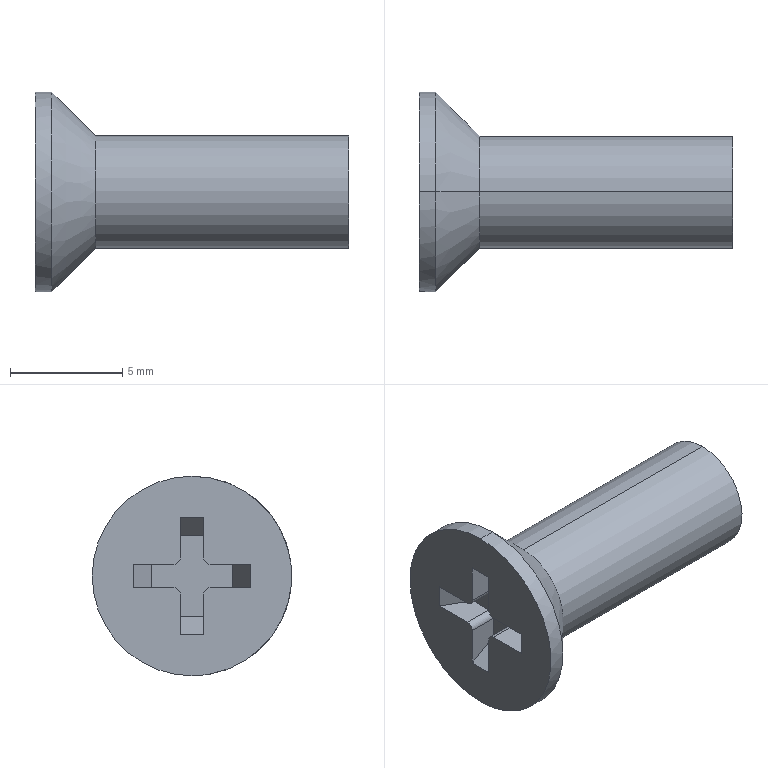Part | STEP file | 46A-01001LS14_Default<As Machined> | 1 solid | 25 faces | box 14 x 8.9 x 8.9 mm | volume 333.383 mm3 | plane 15 | cylinder 8 | cone 2 | commonest cylinder face diameters 0.6 x4 5 x2 8.9 x2
STEP:
#1=CARTESIAN_POINT('',(2.7,0.,-2.5));
#2=VERTEX_POINT('',#1);
#3=CARTESIAN_POINT('',(2.7,0.,2.5));
#4=VERTEX_POINT('',#3);
#5=CARTESIAN_POINT('',(2.7,0.,0.));
#6=DIRECTION('',(1.,0.,0.));
#7=AXIS2_PLACEMENT_3D('',#5,#6,$);
#8=CIRCLE('',#7,2.5);
#9=EDGE_CURVE('',#2,#4,#8,.T.);
#10=ORIENTED_EDGE('',*,*,#9,.T.);
#11=CARTESIAN_POINT('',(14.,0.,2.5));
#12=VERTEX_POINT('',#11);
#13=CARTESIAN_POINT('',(4.516,0.,2.5));
#14=DIRECTION('',(1.,0.,0.));
#15=VECTOR('',#14,1.);
#16=LINE('',#13,#15);
#17=EDGE_CURVE('',#4,#12,#16,.T.);
#18=ORIENTED_EDGE('',*,*,#17,.T.);
#19=CARTESIAN_POINT('',(14.,0.,-2.5));
#20=VERTEX_POINT('',#19);
#21=CARTESIAN_POINT('',(14.,0.,0.));
#22=DIRECTION('',(1.,0.,0.));
#23=AXIS2_PLACEMENT_3D('',#21,#22,$);
#24=CIRCLE('',#23,2.5);
#25=EDGE_CURVE('',#20,#12,#24,.T.);
#26=ORIENTED_EDGE('',*,*,#25,.F.);
#27=CARTESIAN_POINT('',(4.516,0.,-2.5));
#28=DIRECTION('',(1.,0.,0.));
#29=VECTOR('',#28,1.);
#30=LINE('',#27,#29);
#31=EDGE_CURVE('',#2,#20,#30,.T.);
#32=ORIENTED_EDGE('',*,*,#31,.F.);
#33=EDGE_LOOP('',(#10,#18,#26,#32));
#34=FACE_OUTER_BOUND('',#33,.T.);
#35=CARTESIAN_POINT('',(4.516,0.,0.));
#36=DIRECTION('',(1.,0.,0.));
#37=DIRECTION('',(0.,0.,-1.));
#38=AXIS2_PLACEMENT_3D('',#35,#36,#37);
#39=CYLINDRICAL_SURFACE('',#38,2.5);
#40=ADVANCED_FACE('',(#34),#39,.T.);
#41=ORIENTED_EDGE('',*,*,#9,.F.);
#42=CARTESIAN_POINT('',(0.75,0.,-4.45));
#43=VERTEX_POINT('',#42);
#44=CARTESIAN_POINT('',(-353549.441,0.,-353554.641));
#45=DIRECTION('',(-0.7071,0.,-0.7071));
#46=VECTOR('',#45,1.);
#47=LINE('',#44,#46);
#48=EDGE_CURVE('',#2,#43,#47,.T.);
#49=ORIENTED_EDGE('',*,*,#48,.T.);
#50=CARTESIAN_POINT('',(0.75,0.,4.45));
#51=VERTEX_POINT('',#50);
#52=CARTESIAN_POINT('',(0.75,0.,0.));
#53=DIRECTION('',(-1.,0.,0.));
#54=AXIS2_PLACEMENT_3D('',#52,#53,$);
#55=CIRCLE('',#54,4.45);
#56=EDGE_CURVE('',#43,#51,#55,.F.);
#57=ORIENTED_EDGE('',*,*,#56,.T.);
#58=CARTESIAN_POINT('',(-353549.441,0.,353554.641));
#59=DIRECTION('',(-0.7071,0.,0.7071));
#60=VECTOR('',#59,1.);
#61=LINE('',#58,#60);
#62=EDGE_CURVE('',#4,#51,#61,.T.);
#63=ORIENTED_EDGE('',*,*,#62,.F.);
#64=EDGE_LOOP('',(#41,#49,#57,#63));
#65=FACE_OUTER_BOUND('',#64,.T.);
#66=CARTESIAN_POINT('',(2.7,0.,0.));
#67=DIRECTION('',(-1.,0.,0.));
#68=DIRECTION('',(0.,0.,1.));
#69=AXIS2_PLACEMENT_3D('',#66,#67,#68);
#70=CONICAL_SURFACE('',#69,2.5,0.7854);
#71=ADVANCED_FACE('',(#65),#70,.T.);
#72=ORIENTED_EDGE('',*,*,#17,.F.);
#73=CARTESIAN_POINT('',(2.7,0.,2.5));
#74=CARTESIAN_POINT('',(2.7,-0.7854,2.5));
#75=CARTESIAN_POINT('',(2.7,-1.571,2.192));
#76=CARTESIAN_POINT('',(2.7,-2.192,1.571));
#77=CARTESIAN_POINT('',(2.7,-2.808,0.));
#78=CARTESIAN_POINT('',(2.7,-2.192,-1.571));
#79=CARTESIAN_POINT('',(2.7,-1.571,-2.192));
#80=CARTESIAN_POINT('',(2.7,-0.7854,-2.5));
#81=CARTESIAN_POINT('',(2.7,0.,-2.5));
#82=B_SPLINE_CURVE_WITH_KNOTS('',5,(#73,#74,#75,#76,#77,#78,#79,#80,#81),.UNSPECIFIED.,.F.,.U.,(6,3,6),(-3.927,0.,3.927),.UNSPECIFIED.);
#83=EDGE_CURVE('',#4,#2,#82,.T.);
#84=ORIENTED_EDGE('',*,*,#83,.T.);
#85=ORIENTED_EDGE('',*,*,#31,.T.);
#86=CARTESIAN_POINT('',(14.,0.,2.5));
#87=CARTESIAN_POINT('',(14.,-0.7854,2.5));
#88=CARTESIAN_POINT('',(14.,-1.571,2.192));
#89=CARTESIAN_POINT('',(14.,-2.192,1.571));
#90=CARTESIAN_POINT('',(14.,-2.808,0.));
#91=CARTESIAN_POINT('',(14.,-2.192,-1.571));
#92=CARTESIAN_POINT('',(14.,-1.571,-2.192));
#93=CARTESIAN_POINT('',(14.,-0.7854,-2.5));
#94=CARTESIAN_POINT('',(14.,0.,-2.5));
#95=B_SPLINE_CURVE_WITH_KNOTS('',5,(#86,#87,#88,#89,#90,#91,#92,#93,#94),.UNSPECIFIED.,.F.,.U.,(6,3,6),(-3.927,0.,3.927),.UNSPECIFIED.);
#96=EDGE_CURVE('',#12,#20,#95,.T.);
#97=ORIENTED_EDGE('',*,*,#96,.F.);
#98=EDGE_LOOP('',(#72,#84,#85,#97));
#99=FACE_OUTER_BOUND('',#98,.T.);
#100=CARTESIAN_POINT('',(4.516,0.,0.));
#101=DIRECTION('',(1.,0.,0.));
#102=DIRECTION('',(0.,0.,1.));
#103=AXIS2_PLACEMENT_3D('',#100,#101,#102);
#104=CYLINDRICAL_SURFACE('',#103,2.5);
#105=ADVANCED_FACE('',(#99),#104,.T.);
#106=ORIENTED_EDGE('',*,*,#25,.T.);
#107=ORIENTED_EDGE('',*,*,#96,.T.);
#108=EDGE_LOOP('',(#106,#107));
#109=FACE_OUTER_BOUND('',#108,.T.);
#110=CARTESIAN_POINT('',(14.,2.5,0.));
#111=DIRECTION('',(1.,0.,0.));
#112=DIRECTION('',(0.,0.,-1.));
#113=AXIS2_PLACEMENT_3D('',#110,#111,#112);
#114=PLANE('',#113);
#115=ADVANCED_FACE('',(#109),#114,.T.);
#116=ORIENTED_EDGE('',*,*,#48,.F.);
#117=ORIENTED_EDGE('',*,*,#83,.F.);
#118=ORIENTED_EDGE('',*,*,#62,.T.);
#119=CARTESIAN_POINT('',(0.75,0.,0.));
#120=DIRECTION('',(-1.,0.,0.));
#121=AXIS2_PLACEMENT_3D('',#119,#120,$);
#122=CIRCLE('',#121,4.45);
#123=EDGE_CURVE('',#51,#43,#122,.F.);
#124=ORIENTED_EDGE('',*,*,#123,.T.);
#125=EDGE_LOOP('',(#116,#117,#118,#124));
#126=FACE_OUTER_BOUND('',#125,.T.);
#127=CARTESIAN_POINT('',(2.7,0.,0.));
#128=DIRECTION('',(-1.,0.,0.));
#129=DIRECTION('',(0.,0.,-1.));
#130=AXIS2_PLACEMENT_3D('',#127,#128,#129);
#131=CONICAL_SURFACE('',#130,2.5,0.7854);
#132=ADVANCED_FACE('',(#126),#131,.T.);
#133=CARTESIAN_POINT('',(0.,0.,-4.45));
#134=VERTEX_POINT('',#133);
#135=CARTESIAN_POINT('',(0.,0.,4.45));
#136=VERTEX_POINT('',#135);
#137=CARTESIAN_POINT('',(0.,0.,0.));
#138=DIRECTION('',(1.,0.,0.));
#139=AXIS2_PLACEMENT_3D('',#137,#138,$);
#140=CIRCLE('',#139,4.45);
#141=EDGE_CURVE('',#134,#136,#140,.T.);
#142=ORIENTED_EDGE('',*,*,#141,.T.);
#143=CARTESIAN_POINT('',(4.516,0.,4.45));
#144=DIRECTION('',(1.,0.,0.));
#145=VECTOR('',#144,1.);
#146=LINE('',#143,#145);
#147=EDGE_CURVE('',#136,#51,#146,.T.);
#148=ORIENTED_EDGE('',*,*,#147,.T.);
#149=ORIENTED_EDGE('',*,*,#56,.F.);
#150=CARTESIAN_POINT('',(4.516,0.,-4.45));
#151=DIRECTION('',(1.,0.,0.));
#152=VECTOR('',#151,1.);
#153=LINE('',#150,#152);
#154=EDGE_CURVE('',#134,#43,#153,.T.);
#155=ORIENTED_EDGE('',*,*,#154,.F.);
#156=EDGE_LOOP('',(#142,#148,#149,#155));
#157=FACE_OUTER_BOUND('',#156,.T.);
#158=CARTESIAN_POINT('',(4.516,0.,0.));
#159=DIRECTION('',(1.,0.,0.));
#160=DIRECTION('',(0.,0.,-1.));
#161=AXIS2_PLACEMENT_3D('',#158,#159,#160);
#162=CYLINDRICAL_SURFACE('',#161,4.45);
#163=ADVANCED_FACE('',(#157),#162,.T.);
#164=ORIENTED_EDGE('',*,*,#147,.F.);
#165=CARTESIAN_POINT('',(0.,0.,4.45));
#166=CARTESIAN_POINT('',(0.,-0.699,4.45));
#167=CARTESIAN_POINT('',(0.,-1.398,4.313));
#168=CARTESIAN_POINT('',(0.,-2.061,4.038));
#169=CARTESIAN_POINT('',(0.,-3.244,3.244));
#170=CARTESIAN_POINT('',(0.,-4.038,2.061));
#171=CARTESIAN_POINT('',(0.,-4.313,1.398));
#172=CARTESIAN_POINT('',(0.,-4.587,0.));
#173=CARTESIAN_POINT('',(0.,-4.313,-1.398));
#174=CARTESIAN_POINT('',(0.,-4.038,-2.061));
#175=CARTESIAN_POINT('',(0.,-3.244,-3.244));
#176=CARTESIAN_POINT('',(0.,-2.061,-4.038));
#177=CARTESIAN_POINT('',(0.,-1.398,-4.313));
#178=CARTESIAN_POINT('',(0.,-0.699,-4.45));
#179=CARTESIAN_POINT('',(0.,0.,-4.45));
#180=B_SPLINE_CURVE_WITH_KNOTS('',5,(#165,#166,#167,#168,#169,#170,#171,#172,#173,#174,#175,#176,#177,#178,#179),.UNSPECIFIED.,.F.,.U.,(6,3,3,3,6),(-6.99,-3.495,0.,3.495,6.99),.UNSPECIFIED.);
#181=EDGE_CURVE('',#136,#134,#180,.T.);
#182=ORIENTED_EDGE('',*,*,#181,.T.);
#183=ORIENTED_EDGE('',*,*,#154,.T.);
#184=ORIENTED_EDGE('',*,*,#123,.F.);
#185=EDGE_LOOP('',(#164,#182,#183,#184));
#186=FACE_OUTER_BOUND('',#185,.T.);
#187=CARTESIAN_POINT('',(4.516,0.,0.));
#188=DIRECTION('',(1.,0.,0.));
#189=DIRECTION('',(0.,0.,1.));
#190=AXIS2_PLACEMENT_3D('',#187,#188,#189);
#191=CYLINDRICAL_SURFACE('',#190,4.45);
#192=ADVANCED_FACE('',(#186),#191,.T.);
#193=ORIENTED_EDGE('',*,*,#141,.F.);
#194=ORIENTED_EDGE('',*,*,#181,.F.);
#195=EDGE_LOOP('',(#193,#194));
#196=FACE_OUTER_BOUND('',#195,.T.);
#197=CARTESIAN_POINT('',(0.,-2.6,-0.52));
#198=VERTEX_POINT('',#197);
#199=CARTESIAN_POINT('',(0.,-0.82,-0.52));
#200=VERTEX_POINT('',#199);
#201=CARTESIAN_POINT('',(0.,-1.71,-0.52));
#202=DIRECTION('',(0.,1.,0.));
#203=VECTOR('',#202,1.);
#204=LINE('',#201,#203);
#205=EDGE_CURVE('',#198,#200,#204,.T.);
#206=ORIENTED_EDGE('',*,*,#205,.T.);
#207=CARTESIAN_POINT('',(0.,-0.52,-0.82));
#208=VERTEX_POINT('',#207);
#209=CARTESIAN_POINT('',(0.,-0.82,-0.82));
#210=DIRECTION('',(-1.,0.,0.));
#211=AXIS2_PLACEMENT_3D('',#209,#210,$);
#212=CIRCLE('',#211,0.3);
#213=EDGE_CURVE('',#200,#208,#212,.T.);
#214=ORIENTED_EDGE('',*,*,#213,.T.);
#215=CARTESIAN_POINT('',(0.,-0.52,-2.6));
#216=VERTEX_POINT('',#215);
#217=CARTESIAN_POINT('',(0.,-0.52,-1.71));
#218=DIRECTION('',(0.,0.,-1.));
#219=VECTOR('',#218,1.);
#220=LINE('',#217,#219);
#221=EDGE_CURVE('',#208,#216,#220,.T.);
#222=ORIENTED_EDGE('',*,*,#221,.T.);
#223=CARTESIAN_POINT('',(0.,0.52,-2.6));
#224=VERTEX_POINT('',#223);
#225=CARTESIAN_POINT('',(0.,0.,-2.6));
#226=DIRECTION('',(0.,1.,0.));
#227=VECTOR('',#226,1.);
#228=LINE('',#225,#227);
#229=EDGE_CURVE('',#216,#224,#228,.T.);
#230=ORIENTED_EDGE('',*,*,#229,.T.);
#231=CARTESIAN_POINT('',(0.,0.52,-0.82));
#232=VERTEX_POINT('',#231);
#233=CARTESIAN_POINT('',(0.,0.52,-1.71));
#234=DIRECTION('',(0.,0.,1.));
#235=VECTOR('',#234,1.);
#236=LINE('',#233,#235);
#237=EDGE_CURVE('',#224,#232,#236,.T.);
#238=ORIENTED_EDGE('',*,*,#237,.T.);
#239=CARTESIAN_POINT('',(0.,0.82,-0.52));
#240=VERTEX_POINT('',#239);
#241=CARTESIAN_POINT('',(0.,0.82,-0.82));
#242=DIRECTION('',(-1.,0.,0.));
#243=AXIS2_PLACEMENT_3D('',#241,#242,$);
#244=CIRCLE('',#243,0.3);
#245=EDGE_CURVE('',#232,#240,#244,.T.);
#246=ORIENTED_EDGE('',*,*,#245,.T.);
#247=CARTESIAN_POINT('',(0.,2.6,-0.52));
#248=VERTEX_POINT('',#247);
#249=CARTESIAN_POINT('',(0.,1.71,-0.52));
#250=DIRECTION('',(0.,1.,0.));
#251=VECTOR('',#250,1.);
#252=LINE('',#249,#251);
#253=EDGE_CURVE('',#240,#248,#252,.T.);
#254=ORIENTED_EDGE('',*,*,#253,.T.);
#255=CARTESIAN_POINT('',(0.,2.6,0.52));
#256=VERTEX_POINT('',#255);
#257=CARTESIAN_POINT('',(0.,2.6,0.));
#258=DIRECTION('',(0.,0.,1.));
#259=VECTOR('',#258,1.);
#260=LINE('',#257,#259);
#261=EDGE_CURVE('',#248,#256,#260,.T.);
#262=ORIENTED_EDGE('',*,*,#261,.T.);
#263=CARTESIAN_POINT('',(0.,0.82,0.52));
#264=VERTEX_POINT('',#263);
#265=CARTESIAN_POINT('',(0.,1.71,0.52));
#266=DIRECTION('',(0.,-1.,0.));
#267=VECTOR('',#266,1.);
#268=LINE('',#265,#267);
#269=EDGE_CURVE('',#256,#264,#268,.T.);
#270=ORIENTED_EDGE('',*,*,#269,.T.);
#271=CARTESIAN_POINT('',(0.,0.52,0.82));
#272=VERTEX_POINT('',#271);
#273=CARTESIAN_POINT('',(0.,0.82,0.82));
#274=DIRECTION('',(-1.,0.,0.));
#275=AXIS2_PLACEMENT_3D('',#273,#274,$);
#276=CIRCLE('',#275,0.3);
#277=EDGE_CURVE('',#264,#272,#276,.T.);
#278=ORIENTED_EDGE('',*,*,#277,.T.);
#279=CARTESIAN_POINT('',(0.,0.52,2.6));
#280=VERTEX_POINT('',#279);
#281=CARTESIAN_POINT('',(0.,0.52,1.71));
#282=DIRECTION('',(0.,0.,1.));
#283=VECTOR('',#282,1.);
#284=LINE('',#281,#283);
#285=EDGE_CURVE('',#272,#280,#284,.T.);
#286=ORIENTED_EDGE('',*,*,#285,.T.);
#287=CARTESIAN_POINT('',(0.,-0.52,2.6));
#288=VERTEX_POINT('',#287);
#289=CARTESIAN_POINT('',(0.,0.,2.6));
#290=DIRECTION('',(0.,-1.,0.));
#291=VECTOR('',#290,1.);
#292=LINE('',#289,#291);
#293=EDGE_CURVE('',#280,#288,#292,.T.);
#294=ORIENTED_EDGE('',*,*,#293,.T.);
#295=CARTESIAN_POINT('',(0.,-0.52,0.82));
#296=VERTEX_POINT('',#295);
#297=CARTESIAN_POINT('',(0.,-0.52,1.71));
#298=DIRECTION('',(0.,0.,-1.));
#299=VECTOR('',#298,1.);
#300=LINE('',#297,#299);
#301=EDGE_CURVE('',#288,#296,#300,.T.);
#302=ORIENTED_EDGE('',*,*,#301,.T.);
#303=CARTESIAN_POINT('',(0.,-0.82,0.52));
#304=VERTEX_POINT('',#303);
#305=CARTESIAN_POINT('',(0.,-0.82,0.82));
#306=DIRECTION('',(-1.,0.,0.));
#307=AXIS2_PLACEMENT_3D('',#305,#306,$);
#308=CIRCLE('',#307,0.3);
#309=EDGE_CURVE('',#296,#304,#308,.T.);
#310=ORIENTED_EDGE('',*,*,#309,.T.);
#311=CARTESIAN_POINT('',(0.,-2.6,0.52));
#312=VERTEX_POINT('',#311);
#313=CARTESIAN_POINT('',(0.,-1.71,0.52));
#314=DIRECTION('',(0.,-1.,0.));
#315=VECTOR('',#314,1.);
#316=LINE('',#313,#315);
#317=EDGE_CURVE('',#304,#312,#316,.T.);
#318=ORIENTED_EDGE('',*,*,#317,.T.);
#319=CARTESIAN_POINT('',(0.,-2.6,0.));
#320=DIRECTION('',(0.,0.,-1.));
#321=VECTOR('',#320,1.);
#322=LINE('',#319,#321);
#323=EDGE_CURVE('',#312,#198,#322,.T.);
#324=ORIENTED_EDGE('',*,*,#323,.T.);
#325=EDGE_LOOP('',(#206,#214,#222,#230,#238,#246,#254,#262,#270,#278,#286,#294,#302,#310,#318,#324));
#326=FACE_BOUND('',#325,.T.);
#327=CARTESIAN_POINT('',(0.,4.45,0.));
#328=DIRECTION('',(-1.,0.,0.));
#329=DIRECTION('',(0.,0.,1.));
#330=AXIS2_PLACEMENT_3D('',#327,#328,#329);
#331=PLANE('',#330);
#332=ADVANCED_FACE('',(#196,#326),#331,.T.);
#333=CARTESIAN_POINT('',(1.35,-1.821,-0.52));
#334=VERTEX_POINT('',#333);
#335=CARTESIAN_POINT('',(1.35,-0.82,-0.52));
#336=VERTEX_POINT('',#335);
#337=CARTESIAN_POINT('',(1.35,-1.32,-0.52));
#338=DIRECTION('',(0.,1.,0.));
#339=VECTOR('',#338,1.);
#340=LINE('',#337,#339);
#341=EDGE_CURVE('',#334,#336,#340,.T.);
#342=ORIENTED_EDGE('',*,*,#341,.T.);
#343=CARTESIAN_POINT('',(0.675,-0.82,-0.52));
#344=DIRECTION('',(-1.,0.,0.));
#345=VECTOR('',#344,1.);
#346=LINE('',#343,#345);
#347=EDGE_CURVE('',#336,#200,#346,.T.);
#348=ORIENTED_EDGE('',*,*,#347,.T.);
#349=ORIENTED_EDGE('',*,*,#205,.F.);
#350=CARTESIAN_POINT('',(0.675,-2.21,-0.52));
#351=DIRECTION('',(-0.866,-0.5,0.));
#352=VECTOR('',#351,1.);
#353=LINE('',#350,#352);
#354=EDGE_CURVE('',#334,#198,#353,.T.);
#355=ORIENTED_EDGE('',*,*,#354,.F.);
#356=EDGE_LOOP('',(#342,#348,#349,#355));
#357=FACE_OUTER_BOUND('',#356,.T.);
#358=CARTESIAN_POINT('',(1.35,-0.52,-0.52));
#359=DIRECTION('',(0.,0.,1.));
#360=DIRECTION('',(1.,0.,0.));
#361=AXIS2_PLACEMENT_3D('',#358,#359,#360);
#362=PLANE('',#361);
#363=ADVANCED_FACE('',(#357),#362,.T.);
#364=CARTESIAN_POINT('',(1.35,-0.52,-0.82));
#365=VERTEX_POINT('',#364);
#366=CARTESIAN_POINT('',(1.35,-0.82,-0.82));
#367=DIRECTION('',(-1.,0.,0.));
#368=AXIS2_PLACEMENT_3D('',#366,#367,$);
#369=CIRCLE('',#368,0.3);
#370=EDGE_CURVE('',#365,#336,#369,.F.);
#371=ORIENTED_EDGE('',*,*,#370,.F.);
#372=CARTESIAN_POINT('',(1.35,-0.52,-0.82));
#373=DIRECTION('',(-1.,0.,0.));
#374=VECTOR('',#373,1.);
#375=LINE('',#372,#374);
#376=EDGE_CURVE('',#208,#365,#375,.F.);
#377=ORIENTED_EDGE('',*,*,#376,.F.);
#378=ORIENTED_EDGE('',*,*,#213,.F.);
#379=ORIENTED_EDGE('',*,*,#347,.F.);
#380=EDGE_LOOP('',(#371,#377,#378,#379));
#381=FACE_OUTER_BOUND('',#380,.T.);
#382=CARTESIAN_POINT('',(1.35,-0.82,-0.82));
#383=DIRECTION('',(-1.,0.,0.));
#384=DIRECTION('',(0.,0.,1.));
#385=AXIS2_PLACEMENT_3D('',#382,#383,#384);
#386=CYLINDRICAL_SURFACE('',#385,0.3);
#387=ADVANCED_FACE('',(#381),#386,.T.);
#388=ORIENTED_EDGE('',*,*,#221,.F.);
#389=ORIENTED_EDGE('',*,*,#376,.T.);
#390=CARTESIAN_POINT('',(1.35,-0.52,-1.821));
#391=VERTEX_POINT('',#390);
#392=CARTESIAN_POINT('',(1.35,-0.52,-1.32));
#393=DIRECTION('',(0.,0.,-1.));
#394=VECTOR('',#393,1.);
#395=LINE('',#392,#394);
#396=EDGE_CURVE('',#365,#391,#395,.T.);
#397=ORIENTED_EDGE('',*,*,#396,.T.);
#398=CARTESIAN_POINT('',(0.675,-0.52,-2.21));
#399=DIRECTION('',(-0.866,0.,-0.5));
#400=VECTOR('',#399,1.);
#401=LINE('',#398,#400);
#402=EDGE_CURVE('',#391,#216,#401,.T.);
#403=ORIENTED_EDGE('',*,*,#402,.T.);
#404=EDGE_LOOP('',(#388,#389,#397,#403));
#405=FACE_OUTER_BOUND('',#404,.T.);
#406=CARTESIAN_POINT('',(1.35,-0.52,-0.52));
#407=DIRECTION('',(0.,1.,0.));
#408=DIRECTION('',(0.,0.,1.));
#409=AXIS2_PLACEMENT_3D('',#406,#407,#408);
#410=PLANE('',#409);
#411=ADVANCED_FACE('',(#405),#410,.T.);
#412=ORIENTED_EDGE('',*,*,#229,.F.);
#413=ORIENTED_EDGE('',*,*,#402,.F.);
#414=CARTESIAN_POINT('',(1.35,0.52,-1.821));
#415=VERTEX_POINT('',#414);
#416=CARTESIAN_POINT('',(1.35,0.,-1.821));
#417=DIRECTION('',(0.,1.,0.));
#418=VECTOR('',#417,1.);
#419=LINE('',#416,#418);
#420=EDGE_CURVE('',#391,#415,#419,.T.);
#421=ORIENTED_EDGE('',*,*,#420,.T.);
#422=CARTESIAN_POINT('',(0.675,0.52,-2.21));
#423=DIRECTION('',(-0.866,0.,-0.5));
#424=VECTOR('',#423,1.);
#425=LINE('',#422,#424);
#426=EDGE_CURVE('',#415,#224,#425,.T.);
#427=ORIENTED_EDGE('',*,*,#426,.T.);
#428=EDGE_LOOP('',(#412,#413,#421,#427));
#429=FACE_OUTER_BOUND('',#428,.T.);
#430=CARTESIAN_POINT('',(0.,0.52,-2.6));
#431=DIRECTION('',(-0.5,0.,0.866));
#432=DIRECTION('',(0.866,0.,0.5));
#433=AXIS2_PLACEMENT_3D('',#430,#431,#432);
#434=PLANE('',#433);
#435=ADVANCED_FACE('',(#429),#434,.T.);
#436=CARTESIAN_POINT('',(1.35,0.52,-0.82));
#437=VERTEX_POINT('',#436);
#438=CARTESIAN_POINT('',(1.35,0.52,-1.32));
#439=DIRECTION('',(0.,0.,1.));
#440=VECTOR('',#439,1.);
#441=LINE('',#438,#440);
#442=EDGE_CURVE('',#415,#437,#441,.T.);
#443=ORIENTED_EDGE('',*,*,#442,.T.);
#444=CARTESIAN_POINT('',(0.675,0.52,-0.82));
#445=DIRECTION('',(-1.,0.,0.));
#446=VECTOR('',#445,1.);
#447=LINE('',#444,#446);
#448=EDGE_CURVE('',#437,#232,#447,.T.);
#449=ORIENTED_EDGE('',*,*,#448,.T.);
#450=ORIENTED_EDGE('',*,*,#237,.F.);
#451=ORIENTED_EDGE('',*,*,#426,.F.);
#452=EDGE_LOOP('',(#443,#449,#450,#451));
#453=FACE_OUTER_BOUND('',#452,.T.);
#454=CARTESIAN_POINT('',(1.35,0.52,-0.52));
#455=DIRECTION('',(0.,-1.,0.));
#456=DIRECTION('',(0.,0.,-1.));
#457=AXIS2_PLACEMENT_3D('',#454,#455,#456);
#458=PLANE('',#457);
#459=ADVANCED_FACE('',(#453),#458,.T.);
#460=CARTESIAN_POINT('',(1.35,0.82,-0.52));
#461=VERTEX_POINT('',#460);
#462=CARTESIAN_POINT('',(1.35,0.82,-0.82));
#463=DIRECTION('',(-1.,0.,0.));
#464=AXIS2_PLACEMENT_3D('',#462,#463,$);
#465=CIRCLE('',#464,0.3);
#466=EDGE_CURVE('',#461,#437,#465,.F.);
#467=ORIENTED_EDGE('',*,*,#466,.F.);
#468=CARTESIAN_POINT('',(1.35,0.82,-0.52));
#469=DIRECTION('',(-1.,0.,0.));
#470=VECTOR('',#469,1.);
#471=LINE('',#468,#470);
#472=EDGE_CURVE('',#240,#461,#471,.F.);
#473=ORIENTED_EDGE('',*,*,#472,.F.);
#474=ORIENTED_EDGE('',*,*,#245,.F.);
#475=ORIENTED_EDGE('',*,*,#448,.F.);
#476=EDGE_LOOP('',(#467,#473,#474,#475));
#477=FACE_OUTER_BOUND('',#476,.T.);
#478=CARTESIAN_POINT('',(1.35,0.82,-0.82));
#479=DIRECTION('',(-1.,0.,0.));
#480=DIRECTION('',(0.,0.,-1.));
#481=AXIS2_PLACEMENT_3D('',#478,#479,#480);
#482=CYLINDRICAL_SURFACE('',#481,0.3);
#483=ADVANCED_FACE('',(#477),#482,.T.);
#484=ORIENTED_EDGE('',*,*,#253,.F.);
#485=ORIENTED_EDGE('',*,*,#472,.T.);
#486=CARTESIAN_POINT('',(1.35,1.821,-0.52));
#487=VERTEX_POINT('',#486);
#488=CARTESIAN_POINT('',(1.35,1.32,-0.52));
#489=DIRECTION('',(0.,1.,0.));
#490=VECTOR('',#489,1.);
#491=LINE('',#488,#490);
#492=EDGE_CURVE('',#461,#487,#491,.T.);
#493=ORIENTED_EDGE('',*,*,#492,.T.);
#494=CARTESIAN_POINT('',(0.675,2.21,-0.52));
#495=DIRECTION('',(-0.866,0.5,0.));
#496=VECTOR('',#495,1.);
#497=LINE('',#494,#496);
#498=EDGE_CURVE('',#487,#248,#497,.T.);
#499=ORIENTED_EDGE('',*,*,#498,.T.);
#500=EDGE_LOOP('',(#484,#485,#493,#499));
#501=FACE_OUTER_BOUND('',#500,.T.);
#502=CARTESIAN_POINT('',(1.35,0.52,-0.52));
#503=DIRECTION('',(0.,0.,1.));
#504=DIRECTION('',(1.,0.,0.));
#505=AXIS2_PLACEMENT_3D('',#502,#503,#504);
#506=PLANE('',#505);
#507=ADVANCED_FACE('',(#501),#506,.T.);
#508=ORIENTED_EDGE('',*,*,#261,.F.);
#509=ORIENTED_EDGE('',*,*,#498,.F.);
#510=CARTESIAN_POINT('',(1.35,1.821,0.52));
#511=VERTEX_POINT('',#510);
#512=CARTESIAN_POINT('',(1.35,1.821,0.));
#513=DIRECTION('',(0.,0.,1.));
#514=VECTOR('',#513,1.);
#515=LINE('',#512,#514);
#516=EDGE_CURVE('',#487,#511,#515,.T.);
#517=ORIENTED_EDGE('',*,*,#516,.T.);
#518=CARTESIAN_POINT('',(0.675,2.21,0.52));
#519=DIRECTION('',(-0.866,0.5,0.));
#520=VECTOR('',#519,1.);
#521=LINE('',#518,#520);
#522=EDGE_CURVE('',#511,#256,#521,.T.);
#523=ORIENTED_EDGE('',*,*,#522,.T.);
#524=EDGE_LOOP('',(#508,#509,#517,#523));
#525=FACE_OUTER_BOUND('',#524,.T.);
#526=CARTESIAN_POINT('',(0.,2.6,-0.52));
#527=DIRECTION('',(-0.5,-0.866,0.));
#528=DIRECTION('',(0.866,-0.5,0.));
#529=AXIS2_PLACEMENT_3D('',#526,#527,#528);
#530=PLANE('',#529);
#531=ADVANCED_FACE('',(#525),#530,.T.);
#532=CARTESIAN_POINT('',(1.35,0.82,0.52));
#533=VERTEX_POINT('',#532);
#534=CARTESIAN_POINT('',(1.35,1.32,0.52));
#535=DIRECTION('',(0.,-1.,0.));
#536=VECTOR('',#535,1.);
#537=LINE('',#534,#536);
#538=EDGE_CURVE('',#511,#533,#537,.T.);
#539=ORIENTED_EDGE('',*,*,#538,.T.);
#540=CARTESIAN_POINT('',(0.675,0.82,0.52));
#541=DIRECTION('',(-1.,0.,0.));
#542=VECTOR('',#541,1.);
#543=LINE('',#540,#542);
#544=EDGE_CURVE('',#533,#264,#543,.T.);
#545=ORIENTED_EDGE('',*,*,#544,.T.);
#546=ORIENTED_EDGE('',*,*,#269,.F.);
#547=ORIENTED_EDGE('',*,*,#522,.F.);
#548=EDGE_LOOP('',(#539,#545,#546,#547));
#549=FACE_OUTER_BOUND('',#548,.T.);
#550=CARTESIAN_POINT('',(1.35,0.52,0.52));
#551=DIRECTION('',(0.,0.,-1.));
#552=DIRECTION('',(0.,1.,0.));
#553=AXIS2_PLACEMENT_3D('',#550,#551,#552);
#554=PLANE('',#553);
#555=ADVANCED_FACE('',(#549),#554,.T.);
#556=CARTESIAN_POINT('',(1.35,0.52,0.82));
#557=VERTEX_POINT('',#556);
#558=CARTESIAN_POINT('',(1.35,0.82,0.82));
#559=DIRECTION('',(-1.,0.,0.));
#560=AXIS2_PLACEMENT_3D('',#558,#559,$);
#561=CIRCLE('',#560,0.3);
#562=EDGE_CURVE('',#557,#533,#561,.F.);
#563=ORIENTED_EDGE('',*,*,#562,.F.);
#564=CARTESIAN_POINT('',(1.35,0.52,0.82));
#565=DIRECTION('',(-1.,0.,0.));
#566=VECTOR('',#565,1.);
#567=LINE('',#564,#566);
#568=EDGE_CURVE('',#272,#557,#567,.F.);
#569=ORIENTED_EDGE('',*,*,#568,.F.);
#570=ORIENTED_EDGE('',*,*,#277,.F.);
#571=ORIENTED_EDGE('',*,*,#544,.F.);
#572=EDGE_LOOP('',(#563,#569,#570,#571));
#573=FACE_OUTER_BOUND('',#572,.T.);
#574=CARTESIAN_POINT('',(1.35,0.82,0.82));
#575=DIRECTION('',(-1.,0.,0.));
#576=DIRECTION('',(0.,0.,-1.));
#577=AXIS2_PLACEMENT_3D('',#574,#575,#576);
#578=CYLINDRICAL_SURFACE('',#577,0.3);
#579=ADVANCED_FACE('',(#573),#578,.T.);
#580=ORIENTED_EDGE('',*,*,#285,.F.);
#581=ORIENTED_EDGE('',*,*,#568,.T.);
#582=CARTESIAN_POINT('',(1.35,0.52,1.821));
#583=VERTEX_POINT('',#582);
#584=CARTESIAN_POINT('',(1.35,0.52,1.32));
#585=DIRECTION('',(0.,0.,1.));
#586=VECTOR('',#585,1.);
#587=LINE('',#584,#586);
#588=EDGE_CURVE('',#557,#583,#587,.T.);
#589=ORIENTED_EDGE('',*,*,#588,.T.);
#590=CARTESIAN_POINT('',(0.675,0.52,2.21));
#591=DIRECTION('',(-0.866,0.,0.5));
#592=VECTOR('',#591,1.);
#593=LINE('',#590,#592);
#594=EDGE_CURVE('',#583,#280,#593,.T.);
#595=ORIENTED_EDGE('',*,*,#594,.T.);
#596=EDGE_LOOP('',(#580,#581,#589,#595));
#597=FACE_OUTER_BOUND('',#596,.T.);
#598=CARTESIAN_POINT('',(1.35,0.52,0.52));
#599=DIRECTION('',(0.,-1.,0.));
#600=DIRECTION('',(0.,0.,-1.));
#601=AXIS2_PLACEMENT_3D('',#598,#599,#600);
#602=PLANE('',#601);
#603=ADVANCED_FACE('',(#597),#602,.T.);
#604=ORIENTED_EDGE('',*,*,#293,.F.);
#605=ORIENTED_EDGE('',*,*,#594,.F.);
#606=CARTESIAN_POINT('',(1.35,-0.52,1.821));
#607=VERTEX_POINT('',#606);
#608=CARTESIAN_POINT('',(1.35,0.,1.821));
#609=DIRECTION('',(0.,-1.,0.));
#610=VECTOR('',#609,1.);
#611=LINE('',#608,#610);
#612=EDGE_CURVE('',#583,#607,#611,.T.);
#613=ORIENTED_EDGE('',*,*,#612,.T.);
#614=CARTESIAN_POINT('',(0.675,-0.52,2.21));
#615=DIRECTION('',(-0.866,0.,0.5));
#616=VECTOR('',#615,1.);
#617=LINE('',#614,#616);
#618=EDGE_CURVE('',#607,#288,#617,.T.);
#619=ORIENTED_EDGE('',*,*,#618,.T.);
#620=EDGE_LOOP('',(#604,#605,#613,#619));
#621=FACE_OUTER_BOUND('',#620,.T.);
#622=CARTESIAN_POINT('',(0.,0.52,2.6));
#623=DIRECTION('',(-0.5,0.,-0.866));
#624=DIRECTION('',(-0.866,0.,0.5));
#625=AXIS2_PLACEMENT_3D('',#622,#623,#624);
#626=PLANE('',#625);
#627=ADVANCED_FACE('',(#621),#626,.T.);
#628=CARTESIAN_POINT('',(1.35,-0.52,0.82));
#629=VERTEX_POINT('',#628);
#630=CARTESIAN_POINT('',(1.35,-0.52,1.32));
#631=DIRECTION('',(0.,0.,-1.));
#632=VECTOR('',#631,1.);
#633=LINE('',#630,#632);
#634=EDGE_CURVE('',#607,#629,#633,.T.);
#635=ORIENTED_EDGE('',*,*,#634,.T.);
#636=CARTESIAN_POINT('',(0.675,-0.52,0.82));
#637=DIRECTION('',(-1.,0.,0.));
#638=VECTOR('',#637,1.);
#639=LINE('',#636,#638);
#640=EDGE_CURVE('',#629,#296,#639,.T.);
#641=ORIENTED_EDGE('',*,*,#640,.T.);
#642=ORIENTED_EDGE('',*,*,#301,.F.);
#643=ORIENTED_EDGE('',*,*,#618,.F.);
#644=EDGE_LOOP('',(#635,#641,#642,#643));
#645=FACE_OUTER_BOUND('',#644,.T.);
#646=CARTESIAN_POINT('',(1.35,-0.52,0.52));
#647=DIRECTION('',(0.,1.,0.));
#648=DIRECTION('',(0.,0.,1.));
#649=AXIS2_PLACEMENT_3D('',#646,#647,#648);
#650=PLANE('',#649);
#651=ADVANCED_FACE('',(#645),#650,.T.);
#652=CARTESIAN_POINT('',(1.35,-0.82,0.52));
#653=VERTEX_POINT('',#652);
#654=CARTESIAN_POINT('',(1.35,-0.82,0.82));
#655=DIRECTION('',(-1.,0.,0.));
#656=AXIS2_PLACEMENT_3D('',#654,#655,$);
#657=CIRCLE('',#656,0.3);
#658=EDGE_CURVE('',#653,#629,#657,.F.);
#659=ORIENTED_EDGE('',*,*,#658,.F.);
#660=CARTESIAN_POINT('',(1.35,-0.82,0.52));
#661=DIRECTION('',(-1.,0.,0.));
#662=VECTOR('',#661,1.);
#663=LINE('',#660,#662);
#664=EDGE_CURVE('',#304,#653,#663,.F.);
#665=ORIENTED_EDGE('',*,*,#664,.F.);
#666=ORIENTED_EDGE('',*,*,#309,.F.);
#667=ORIENTED_EDGE('',*,*,#640,.F.);
#668=EDGE_LOOP('',(#659,#665,#666,#667));
#669=FACE_OUTER_BOUND('',#668,.T.);
#670=CARTESIAN_POINT('',(1.35,-0.82,0.82));
#671=DIRECTION('',(-1.,0.,0.));
#672=DIRECTION('',(0.,0.,1.));
#673=AXIS2_PLACEMENT_3D('',#670,#671,#672);
#674=CYLINDRICAL_SURFACE('',#673,0.3);
#675=ADVANCED_FACE('',(#669),#674,.T.);
#676=ORIENTED_EDGE('',*,*,#317,.F.);
#677=ORIENTED_EDGE('',*,*,#664,.T.);
#678=CARTESIAN_POINT('',(1.35,-1.821,0.52));
#679=VERTEX_POINT('',#678);
#680=CARTESIAN_POINT('',(1.35,-1.32,0.52));
#681=DIRECTION('',(0.,-1.,0.));
#682=VECTOR('',#681,1.);
#683=LINE('',#680,#682);
#684=EDGE_CURVE('',#653,#679,#683,.T.);
#685=ORIENTED_EDGE('',*,*,#684,.T.);
#686=CARTESIAN_POINT('',(0.675,-2.21,0.52));
#687=DIRECTION('',(-0.866,-0.5,0.));
#688=VECTOR('',#687,1.);
#689=LINE('',#686,#688);
#690=EDGE_CURVE('',#679,#312,#689,.T.);
#691=ORIENTED_EDGE('',*,*,#690,.T.);
#692=EDGE_LOOP('',(#676,#677,#685,#691));
#693=FACE_OUTER_BOUND('',#692,.T.);
#694=CARTESIAN_POINT('',(1.35,-0.52,0.52));
#695=DIRECTION('',(0.,0.,-1.));
#696=DIRECTION('',(0.,1.,0.));
#697=AXIS2_PLACEMENT_3D('',#694,#695,#696);
#698=PLANE('',#697);
#699=ADVANCED_FACE('',(#693),#698,.T.);
#700=ORIENTED_EDGE('',*,*,#323,.F.);
#701=ORIENTED_EDGE('',*,*,#690,.F.);
#702=CARTESIAN_POINT('',(1.35,-1.821,0.));
#703=DIRECTION('',(0.,0.,-1.));
#704=VECTOR('',#703,1.);
#705=LINE('',#702,#704);
#706=EDGE_CURVE('',#679,#334,#705,.T.);
#707=ORIENTED_EDGE('',*,*,#706,.T.);
#708=ORIENTED_EDGE('',*,*,#354,.T.);
#709=EDGE_LOOP('',(#700,#701,#707,#708));
#710=FACE_OUTER_BOUND('',#709,.T.);
#711=CARTESIAN_POINT('',(0.,-2.6,-0.52));
#712=DIRECTION('',(-0.5,0.866,0.));
#713=DIRECTION('',(-0.866,-0.5,0.));
#714=AXIS2_PLACEMENT_3D('',#711,#712,#713);
#715=PLANE('',#714);
#716=ADVANCED_FACE('',(#710),#715,.T.);
#717=ORIENTED_EDGE('',*,*,#588,.F.);
#718=ORIENTED_EDGE('',*,*,#562,.T.);
#719=ORIENTED_EDGE('',*,*,#538,.F.);
#720=ORIENTED_EDGE('',*,*,#516,.F.);
#721=ORIENTED_EDGE('',*,*,#492,.F.);
#722=ORIENTED_EDGE('',*,*,#466,.T.);
#723=ORIENTED_EDGE('',*,*,#442,.F.);
#724=ORIENTED_EDGE('',*,*,#420,.F.);
#725=ORIENTED_EDGE('',*,*,#396,.F.);
#726=ORIENTED_EDGE('',*,*,#370,.T.);
#727=ORIENTED_EDGE('',*,*,#341,.F.);
#728=ORIENTED_EDGE('',*,*,#706,.F.);
#729=ORIENTED_EDGE('',*,*,#684,.F.);
#730=ORIENTED_EDGE('',*,*,#658,.T.);
#731=ORIENTED_EDGE('',*,*,#634,.F.);
#732=ORIENTED_EDGE('',*,*,#612,.F.);
#733=EDGE_LOOP('',(#717,#718,#719,#720,#721,#722,#723,#724,#725,#726,#727,#728,#729,#730,#731,#732));
#734=FACE_OUTER_BOUND('',#733,.T.);
#735=CARTESIAN_POINT('',(1.35,0.52,0.52));
#736=DIRECTION('',(1.,0.,0.));
#737=DIRECTION('',(0.,0.,-1.));
#738=AXIS2_PLACEMENT_3D('',#735,#736,#737);
#739=PLANE('',#738);
#740=ADVANCED_FACE('',(#734),#739,.F.);
#741=CLOSED_SHELL('',(#40,#71,#105,#115,#132,#163,#192,#332,#363,#387,#411,#435,#459,#483,#507,#531,#555,#579,#603,#627,#651,#675,#699,#716,#740));
#742=MANIFOLD_SOLID_BREP('',#741);
#743=(LENGTH_UNIT()NAMED_UNIT(*)SI_UNIT(.MILLI.,.METRE.));
#744=UNCERTAINTY_MEASURE_WITH_UNIT(LENGTH_MEASURE(0.005),#743,'','');
#745=(NAMED_UNIT(*)PLANE_ANGLE_UNIT()SI_UNIT($,.RADIAN.));
#746=(NAMED_UNIT(*)SI_UNIT($,.STERADIAN.)SOLID_ANGLE_UNIT());
#747=(GEOMETRIC_REPRESENTATION_CONTEXT(3)GLOBAL_UNCERTAINTY_ASSIGNED_CONTEXT((#744))GLOBAL_UNIT_ASSIGNED_CONTEXT((#743,#745,#746))REPRESENTATION_CONTEXT('',''));
#748=ADVANCED_BREP_SHAPE_REPRESENTATION('',(#742),#747);